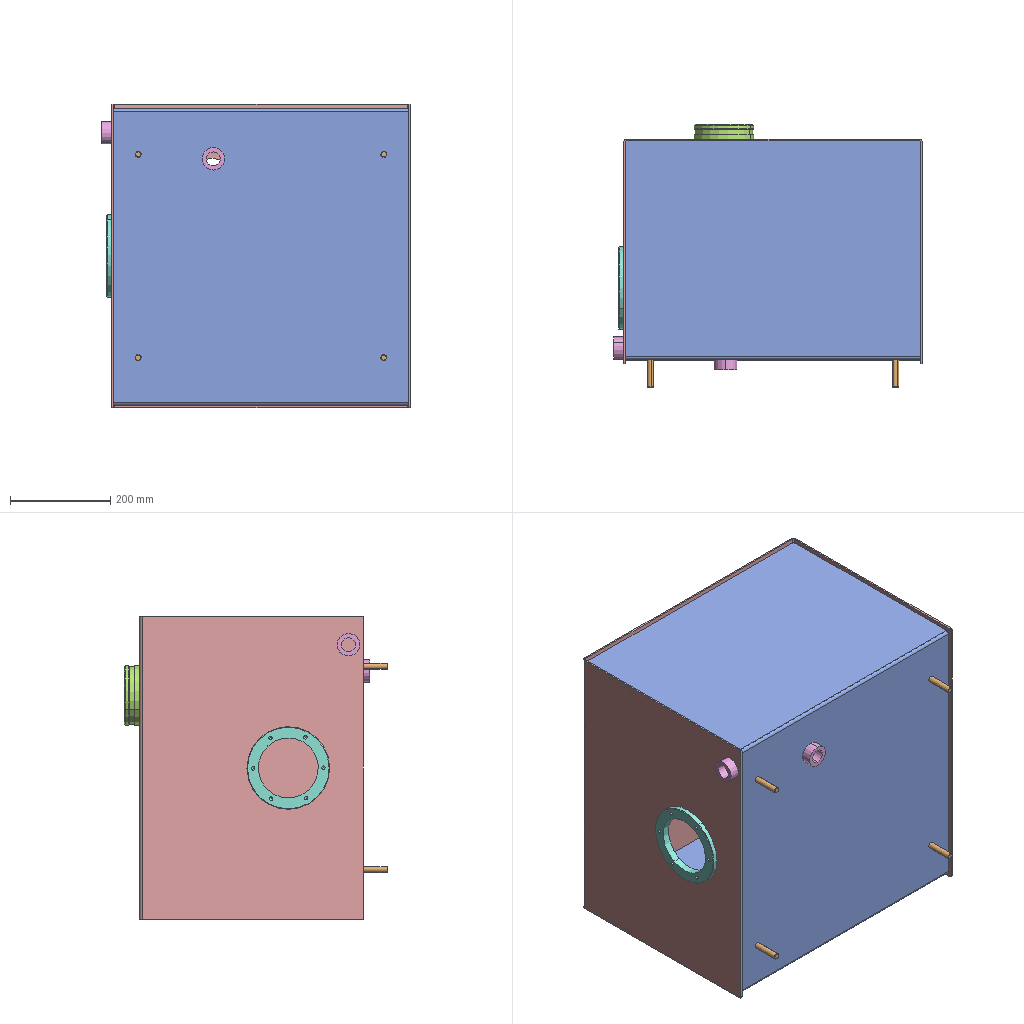Assembly | SolidWorks | 6 different items | 10 placed | box 616 x 525 x 606 mm
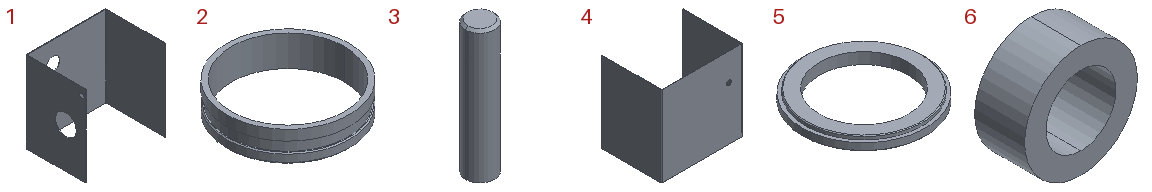Parts list (item | quantity | size | volume | features):
1 | x1 | 596 x 447 x 606 mm | 2607078 mm3 | features ICE 3, FlatPattern 1, SMBaseFlange 1, SheetMetal 1
2 | x1 | 120 x 120 x 30 mm | 45845 mm3 | features Chamfer 2, ICE 2, Extrusion 1
3 | x4 | 12 x 12 x 55 mm | 6203 mm3 | features Chamfer 1, Extrusion 1
4 | x1 | 592 x 437 x 590 mm | 2574453 mm3 | features ICE 2, FlatPattern 1, SMBaseFlange 1, SheetMetal 1
5 | x1 | 165 x 165 x 15 mm | 136481 mm3 | features 3DProfileFeature 1, Chamfer 1, Extrusion 1, HoleWzd 1, ICE 1
6 | x2 | 45 x 23 x 45 mm | 20479 mm3 | features Chamfer 1, Extrusion 1, ICE 1
Mates (type | each side: item.copy, entity, surface, feature):
Coincident | 1.1 face plane Base-Flange1 | 4.1 face plane Base-Flange1 | 2 times
DistanceDim | 4.1 face plane Base-Flange1 | 1.1 face plane Base-Flange1
Coincident | 1.1 face plane Base-Flange1 | 2.1 face plane Boss-Extrude2
Concentric | 1.1 edge | 2.1 edge
Coincident | 4.1 face plane Base-Flange1 | 6.1 face plane Cut-Extrude1
Concentric | 4.1 edge | 6.1 edge
Coincident | 1.1 face plane Base-Flange1 | 6.2 face plane Cut-Extrude1
Concentric | 1.1 edge | 6.2 edge
Coincident | 1.1 face plane Base-Flange1 | 5.1 face plane Boss-Extrude1
Concentric | 1.1 edge | 5.1 edge
Coincident | 4.1 face plane Base-Flange1 | 3.1 face plane Boss-Extrude1
Concentric | 3.1 edge | assembly select_type:10
Coincident | 3.1 face plane Boss-Extrude1 | 3.2 face plane Boss-Extrude1
Coincident | 3.3 face plane Boss-Extrude1 | 3.2 face plane Boss-Extrude1
Coincident | 3.3 face plane Boss-Extrude1 | 3.4 face plane Boss-Extrude1
Concentric | 3.2 edge | assembly select_type:10
Concentric | 3.3 edge | assembly select_type:10
Concentric | 3.4 edge | assembly select_type:10